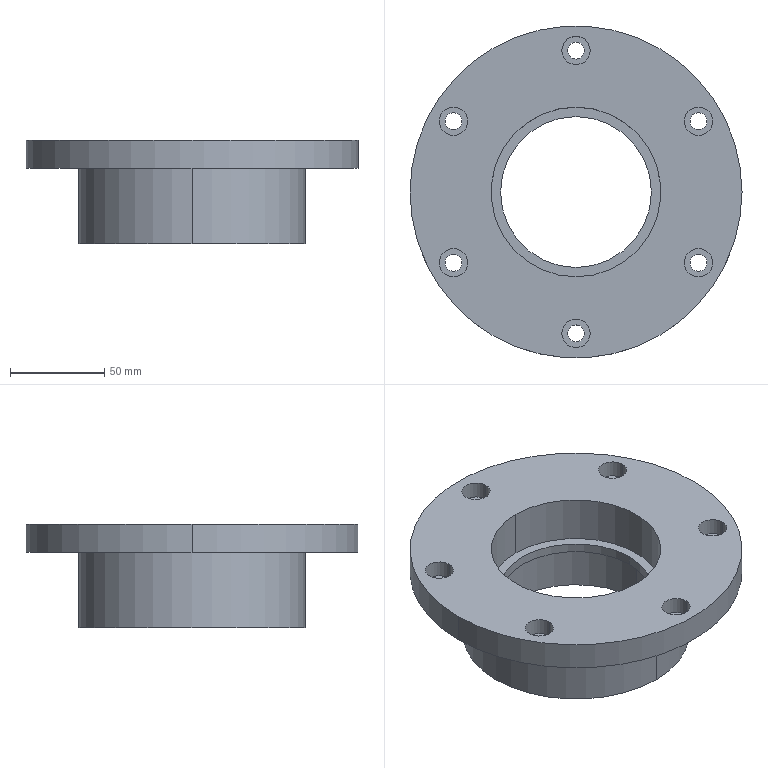Part | SolidWorks | features BaseBody 1 | 1 solid | 45 faces | box 176 x 176 x 55 mm | volume 462265 mm3 | cylinder 34 | plane 11 | commonest cylinder face diameters 9 x12 15 x12 90 x4 80 x2 120 x2 176 x2
STEP:
#1=CARTESIAN_POINT('',(72.452,37.5,46.));
#2=VERTEX_POINT('',#1);
#3=CARTESIAN_POINT('',(57.452,37.5,46.));
#4=VERTEX_POINT('',#3);
#5=CARTESIAN_POINT('',(64.952,37.5,46.));
#6=DIRECTION('',(0.,0.,-1.));
#7=DIRECTION('',(1.,0.,0.));
#8=AXIS2_PLACEMENT_3D('',#5,#6,#7);
#9=CIRCLE('',#8,7.5);
#10=EDGE_CURVE('',#2,#4,#9,.T.);
#11=ORIENTED_EDGE('',*,*,#10,.T.);
#12=CARTESIAN_POINT('',(57.452,37.5,55.));
#13=VERTEX_POINT('',#12);
#14=CARTESIAN_POINT('',(57.452,37.5,46.));
#15=DIRECTION('',(0.,0.,1.));
#16=VECTOR('',#15,1000.);
#17=LINE('',#14,#16);
#18=EDGE_CURVE('',#4,#13,#17,.T.);
#19=ORIENTED_EDGE('',*,*,#18,.T.);
#20=CARTESIAN_POINT('',(72.452,37.5,55.));
#21=VERTEX_POINT('',#20);
#22=CARTESIAN_POINT('',(64.952,37.5,55.));
#23=DIRECTION('',(0.,0.,1.));
#24=DIRECTION('',(1.,0.,0.));
#25=AXIS2_PLACEMENT_3D('',#22,#23,#24);
#26=CIRCLE('',#25,7.5);
#27=EDGE_CURVE('',#13,#21,#26,.T.);
#28=ORIENTED_EDGE('',*,*,#27,.T.);
#29=CARTESIAN_POINT('',(72.452,37.5,46.));
#30=DIRECTION('',(0.,0.,1.));
#31=VECTOR('',#30,1000.);
#32=LINE('',#29,#31);
#33=EDGE_CURVE('',#2,#21,#32,.T.);
#34=ORIENTED_EDGE('',*,*,#33,.F.);
#35=EDGE_LOOP('',(#11,#19,#28,#34));
#36=FACE_OUTER_BOUND('',#35,.T.);
#37=CARTESIAN_POINT('',(64.952,37.5,46.));
#38=DIRECTION('',(0.,0.,1.));
#39=DIRECTION('',(1.,0.,0.));
#40=AXIS2_PLACEMENT_3D('',#37,#38,#39);
#41=CYLINDRICAL_SURFACE('',#40,7.5);
#42=ADVANCED_FACE('',(#36),#41,.F.);
#43=CARTESIAN_POINT('',(0.,-45.,30.));
#44=VERTEX_POINT('',#43);
#45=CARTESIAN_POINT('',(0.,45.,30.));
#46=VERTEX_POINT('',#45);
#47=CARTESIAN_POINT('',(0.,0.,30.));
#48=DIRECTION('',(0.,0.,-1.));
#49=DIRECTION('',(0.,-1.,0.));
#50=AXIS2_PLACEMENT_3D('',#47,#48,#49);
#51=CIRCLE('',#50,45.);
#52=EDGE_CURVE('',#44,#46,#51,.T.);
#53=ORIENTED_EDGE('',*,*,#52,.T.);
#54=CARTESIAN_POINT('',(0.,45.,55.));
#55=VERTEX_POINT('',#54);
#56=CARTESIAN_POINT('',(0.,45.,30.));
#57=DIRECTION('',(0.,0.,1.));
#58=VECTOR('',#57,1000.);
#59=LINE('',#56,#58);
#60=EDGE_CURVE('',#46,#55,#59,.T.);
#61=ORIENTED_EDGE('',*,*,#60,.T.);
#62=CARTESIAN_POINT('',(0.,-45.,55.));
#63=VERTEX_POINT('',#62);
#64=CARTESIAN_POINT('',(0.,0.,55.));
#65=DIRECTION('',(0.,0.,-1.));
#66=DIRECTION('',(0.,-1.,0.));
#67=AXIS2_PLACEMENT_3D('',#64,#65,#66);
#68=CIRCLE('',#67,45.);
#69=EDGE_CURVE('',#63,#55,#68,.T.);
#70=ORIENTED_EDGE('',*,*,#69,.F.);
#71=CARTESIAN_POINT('',(0.,-45.,30.));
#72=DIRECTION('',(0.,0.,1.));
#73=VECTOR('',#72,1000.);
#74=LINE('',#71,#73);
#75=EDGE_CURVE('',#44,#63,#74,.T.);
#76=ORIENTED_EDGE('',*,*,#75,.F.);
#77=EDGE_LOOP('',(#53,#61,#70,#76));
#78=FACE_OUTER_BOUND('',#77,.T.);
#79=CARTESIAN_POINT('',(0.,0.,30.));
#80=DIRECTION('',(0.,0.,1.));
#81=DIRECTION('',(0.,-1.,0.));
#82=AXIS2_PLACEMENT_3D('',#79,#80,#81);
#83=CYLINDRICAL_SURFACE('',#82,45.);
#84=ADVANCED_FACE('',(#78),#83,.F.);
#85=CARTESIAN_POINT('',(7.5,75.,46.));
#86=VERTEX_POINT('',#85);
#87=CARTESIAN_POINT('',(-7.5,75.,46.));
#88=VERTEX_POINT('',#87);
#89=CARTESIAN_POINT('',(0.,75.,46.));
#90=DIRECTION('',(0.,0.,-1.));
#91=DIRECTION('',(1.,0.,0.));
#92=AXIS2_PLACEMENT_3D('',#89,#90,#91);
#93=CIRCLE('',#92,7.5);
#94=EDGE_CURVE('',#86,#88,#93,.T.);
#95=ORIENTED_EDGE('',*,*,#94,.T.);
#96=CARTESIAN_POINT('',(-7.5,75.,55.));
#97=VERTEX_POINT('',#96);
#98=CARTESIAN_POINT('',(-7.5,75.,46.));
#99=DIRECTION('',(0.,0.,1.));
#100=VECTOR('',#99,1000.);
#101=LINE('',#98,#100);
#102=EDGE_CURVE('',#88,#97,#101,.T.);
#103=ORIENTED_EDGE('',*,*,#102,.T.);
#104=CARTESIAN_POINT('',(7.5,75.,55.));
#105=VERTEX_POINT('',#104);
#106=CARTESIAN_POINT('',(0.,75.,55.));
#107=DIRECTION('',(0.,0.,-1.));
#108=DIRECTION('',(1.,0.,0.));
#109=AXIS2_PLACEMENT_3D('',#106,#107,#108);
#110=CIRCLE('',#109,7.5);
#111=EDGE_CURVE('',#105,#97,#110,.T.);
#112=ORIENTED_EDGE('',*,*,#111,.F.);
#113=CARTESIAN_POINT('',(7.5,75.,46.));
#114=DIRECTION('',(0.,0.,1.));
#115=VECTOR('',#114,1000.);
#116=LINE('',#113,#115);
#117=EDGE_CURVE('',#86,#105,#116,.T.);
#118=ORIENTED_EDGE('',*,*,#117,.F.);
#119=EDGE_LOOP('',(#95,#103,#112,#118));
#120=FACE_OUTER_BOUND('',#119,.T.);
#121=CARTESIAN_POINT('',(0.,75.,46.));
#122=DIRECTION('',(0.,0.,1.));
#123=DIRECTION('',(1.,0.,0.));
#124=AXIS2_PLACEMENT_3D('',#121,#122,#123);
#125=CYLINDRICAL_SURFACE('',#124,7.5);
#126=ADVANCED_FACE('',(#120),#125,.F.);
#127=CARTESIAN_POINT('',(-57.452,37.5,46.));
#128=VERTEX_POINT('',#127);
#129=CARTESIAN_POINT('',(-72.452,37.5,46.));
#130=VERTEX_POINT('',#129);
#131=CARTESIAN_POINT('',(-64.952,37.5,46.));
#132=DIRECTION('',(0.,0.,-1.));
#133=DIRECTION('',(1.,0.,0.));
#134=AXIS2_PLACEMENT_3D('',#131,#132,#133);
#135=CIRCLE('',#134,7.5);
#136=EDGE_CURVE('',#128,#130,#135,.T.);
#137=ORIENTED_EDGE('',*,*,#136,.T.);
#138=CARTESIAN_POINT('',(-72.452,37.5,55.));
#139=VERTEX_POINT('',#138);
#140=CARTESIAN_POINT('',(-72.452,37.5,46.));
#141=DIRECTION('',(0.,0.,1.));
#142=VECTOR('',#141,1000.);
#143=LINE('',#140,#142);
#144=EDGE_CURVE('',#130,#139,#143,.T.);
#145=ORIENTED_EDGE('',*,*,#144,.T.);
#146=CARTESIAN_POINT('',(-57.452,37.5,55.));
#147=VERTEX_POINT('',#146);
#148=CARTESIAN_POINT('',(-64.952,37.5,55.));
#149=DIRECTION('',(0.,0.,-1.));
#150=DIRECTION('',(1.,0.,0.));
#151=AXIS2_PLACEMENT_3D('',#148,#149,#150);
#152=CIRCLE('',#151,7.5);
#153=EDGE_CURVE('',#147,#139,#152,.T.);
#154=ORIENTED_EDGE('',*,*,#153,.F.);
#155=CARTESIAN_POINT('',(-57.452,37.5,46.));
#156=DIRECTION('',(0.,0.,1.));
#157=VECTOR('',#156,1000.);
#158=LINE('',#155,#157);
#159=EDGE_CURVE('',#128,#147,#158,.T.);
#160=ORIENTED_EDGE('',*,*,#159,.F.);
#161=EDGE_LOOP('',(#137,#145,#154,#160));
#162=FACE_OUTER_BOUND('',#161,.T.);
#163=CARTESIAN_POINT('',(-64.952,37.5,46.));
#164=DIRECTION('',(0.,0.,1.));
#165=DIRECTION('',(1.,0.,0.));
#166=AXIS2_PLACEMENT_3D('',#163,#164,#165);
#167=CYLINDRICAL_SURFACE('',#166,7.5);
#168=ADVANCED_FACE('',(#162),#167,.F.);
#169=CARTESIAN_POINT('',(-57.452,-37.5,46.));
#170=VERTEX_POINT('',#169);
#171=CARTESIAN_POINT('',(-72.452,-37.5,46.));
#172=VERTEX_POINT('',#171);
#173=CARTESIAN_POINT('',(-64.952,-37.5,46.));
#174=DIRECTION('',(0.,0.,-1.));
#175=DIRECTION('',(1.,0.,0.));
#176=AXIS2_PLACEMENT_3D('',#173,#174,#175);
#177=CIRCLE('',#176,7.5);
#178=EDGE_CURVE('',#170,#172,#177,.T.);
#179=ORIENTED_EDGE('',*,*,#178,.T.);
#180=CARTESIAN_POINT('',(-72.452,-37.5,55.));
#181=VERTEX_POINT('',#180);
#182=CARTESIAN_POINT('',(-72.452,-37.5,46.));
#183=DIRECTION('',(0.,0.,1.));
#184=VECTOR('',#183,1000.);
#185=LINE('',#182,#184);
#186=EDGE_CURVE('',#172,#181,#185,.T.);
#187=ORIENTED_EDGE('',*,*,#186,.T.);
#188=CARTESIAN_POINT('',(-57.452,-37.5,55.));
#189=VERTEX_POINT('',#188);
#190=CARTESIAN_POINT('',(-64.952,-37.5,55.));
#191=DIRECTION('',(0.,0.,-1.));
#192=DIRECTION('',(1.,0.,0.));
#193=AXIS2_PLACEMENT_3D('',#190,#191,#192);
#194=CIRCLE('',#193,7.5);
#195=EDGE_CURVE('',#189,#181,#194,.T.);
#196=ORIENTED_EDGE('',*,*,#195,.F.);
#197=CARTESIAN_POINT('',(-57.452,-37.5,46.));
#198=DIRECTION('',(0.,0.,1.));
#199=VECTOR('',#198,1000.);
#200=LINE('',#197,#199);
#201=EDGE_CURVE('',#170,#189,#200,.T.);
#202=ORIENTED_EDGE('',*,*,#201,.F.);
#203=EDGE_LOOP('',(#179,#187,#196,#202));
#204=FACE_OUTER_BOUND('',#203,.T.);
#205=CARTESIAN_POINT('',(-64.952,-37.5,46.));
#206=DIRECTION('',(0.,0.,1.));
#207=DIRECTION('',(1.,0.,0.));
#208=AXIS2_PLACEMENT_3D('',#205,#206,#207);
#209=CYLINDRICAL_SURFACE('',#208,7.5);
#210=ADVANCED_FACE('',(#204),#209,.F.);
#211=CARTESIAN_POINT('',(7.5,-75.,46.));
#212=VERTEX_POINT('',#211);
#213=CARTESIAN_POINT('',(-7.5,-75.,46.));
#214=VERTEX_POINT('',#213);
#215=CARTESIAN_POINT('',(0.,-75.,46.));
#216=DIRECTION('',(0.,0.,-1.));
#217=DIRECTION('',(1.,0.,0.));
#218=AXIS2_PLACEMENT_3D('',#215,#216,#217);
#219=CIRCLE('',#218,7.5);
#220=EDGE_CURVE('',#212,#214,#219,.T.);
#221=ORIENTED_EDGE('',*,*,#220,.T.);
#222=CARTESIAN_POINT('',(-7.5,-75.,55.));
#223=VERTEX_POINT('',#222);
#224=CARTESIAN_POINT('',(-7.5,-75.,46.));
#225=DIRECTION('',(0.,0.,1.));
#226=VECTOR('',#225,1000.);
#227=LINE('',#224,#226);
#228=EDGE_CURVE('',#214,#223,#227,.T.);
#229=ORIENTED_EDGE('',*,*,#228,.T.);
#230=CARTESIAN_POINT('',(7.5,-75.,55.));
#231=VERTEX_POINT('',#230);
#232=CARTESIAN_POINT('',(0.,-75.,55.));
#233=DIRECTION('',(0.,0.,-1.));
#234=DIRECTION('',(1.,0.,0.));
#235=AXIS2_PLACEMENT_3D('',#232,#233,#234);
#236=CIRCLE('',#235,7.5);
#237=EDGE_CURVE('',#231,#223,#236,.T.);
#238=ORIENTED_EDGE('',*,*,#237,.F.);
#239=CARTESIAN_POINT('',(7.5,-75.,46.));
#240=DIRECTION('',(0.,0.,1.));
#241=VECTOR('',#240,1000.);
#242=LINE('',#239,#241);
#243=EDGE_CURVE('',#212,#231,#242,.T.);
#244=ORIENTED_EDGE('',*,*,#243,.F.);
#245=EDGE_LOOP('',(#221,#229,#238,#244));
#246=FACE_OUTER_BOUND('',#245,.T.);
#247=CARTESIAN_POINT('',(0.,-75.,46.));
#248=DIRECTION('',(0.,0.,1.));
#249=DIRECTION('',(1.,0.,0.));
#250=AXIS2_PLACEMENT_3D('',#247,#248,#249);
#251=CYLINDRICAL_SURFACE('',#250,7.5);
#252=ADVANCED_FACE('',(#246),#251,.F.);
#253=CARTESIAN_POINT('',(72.452,-37.5,46.));
#254=VERTEX_POINT('',#253);
#255=CARTESIAN_POINT('',(57.452,-37.5,46.));
#256=VERTEX_POINT('',#255);
#257=CARTESIAN_POINT('',(64.952,-37.5,46.));
#258=DIRECTION('',(0.,0.,-1.));
#259=DIRECTION('',(1.,0.,0.));
#260=AXIS2_PLACEMENT_3D('',#257,#258,#259);
#261=CIRCLE('',#260,7.5);
#262=EDGE_CURVE('',#254,#256,#261,.T.);
#263=ORIENTED_EDGE('',*,*,#262,.T.);
#264=CARTESIAN_POINT('',(57.452,-37.5,55.));
#265=VERTEX_POINT('',#264);
#266=CARTESIAN_POINT('',(57.452,-37.5,46.));
#267=DIRECTION('',(0.,0.,1.));
#268=VECTOR('',#267,1000.);
#269=LINE('',#266,#268);
#270=EDGE_CURVE('',#256,#265,#269,.T.);
#271=ORIENTED_EDGE('',*,*,#270,.T.);
#272=CARTESIAN_POINT('',(72.452,-37.5,55.));
#273=VERTEX_POINT('',#272);
#274=CARTESIAN_POINT('',(64.952,-37.5,55.));
#275=DIRECTION('',(0.,0.,-1.));
#276=DIRECTION('',(1.,0.,0.));
#277=AXIS2_PLACEMENT_3D('',#274,#275,#276);
#278=CIRCLE('',#277,7.5);
#279=EDGE_CURVE('',#273,#265,#278,.T.);
#280=ORIENTED_EDGE('',*,*,#279,.F.);
#281=CARTESIAN_POINT('',(72.452,-37.5,46.));
#282=DIRECTION('',(0.,0.,1.));
#283=VECTOR('',#282,1000.);
#284=LINE('',#281,#283);
#285=EDGE_CURVE('',#254,#273,#284,.T.);
#286=ORIENTED_EDGE('',*,*,#285,.F.);
#287=EDGE_LOOP('',(#263,#271,#280,#286));
#288=FACE_OUTER_BOUND('',#287,.T.);
#289=CARTESIAN_POINT('',(64.952,-37.5,46.));
#290=DIRECTION('',(0.,0.,1.));
#291=DIRECTION('',(1.,0.,0.));
#292=AXIS2_PLACEMENT_3D('',#289,#290,#291);
#293=CYLINDRICAL_SURFACE('',#292,7.5);
#294=ADVANCED_FACE('',(#288),#293,.F.);
#295=CARTESIAN_POINT('',(88.,0.,55.));
#296=VERTEX_POINT('',#295);
#297=CARTESIAN_POINT('',(-88.,0.,55.));
#298=VERTEX_POINT('',#297);
#299=CARTESIAN_POINT('',(0.,0.,55.));
#300=DIRECTION('',(0.,0.,1.));
#301=DIRECTION('',(-1.,0.,0.));
#302=AXIS2_PLACEMENT_3D('',#299,#300,#301);
#303=CIRCLE('',#302,88.);
#304=EDGE_CURVE('',#296,#298,#303,.T.);
#305=ORIENTED_EDGE('',*,*,#304,.F.);
#306=CARTESIAN_POINT('',(88.,0.,40.));
#307=VERTEX_POINT('',#306);
#308=CARTESIAN_POINT('',(88.,0.,55.));
#309=DIRECTION('',(0.,0.,-1.));
#310=VECTOR('',#309,1000.);
#311=LINE('',#308,#310);
#312=EDGE_CURVE('',#296,#307,#311,.T.);
#313=ORIENTED_EDGE('',*,*,#312,.T.);
#314=CARTESIAN_POINT('',(-88.,0.,40.));
#315=VERTEX_POINT('',#314);
#316=CARTESIAN_POINT('',(0.,0.,40.));
#317=DIRECTION('',(0.,0.,-1.));
#318=DIRECTION('',(-1.,0.,0.));
#319=AXIS2_PLACEMENT_3D('',#316,#317,#318);
#320=CIRCLE('',#319,88.);
#321=EDGE_CURVE('',#315,#307,#320,.T.);
#322=ORIENTED_EDGE('',*,*,#321,.F.);
#323=CARTESIAN_POINT('',(-88.,0.,55.));
#324=DIRECTION('',(0.,0.,-1.));
#325=VECTOR('',#324,1000.);
#326=LINE('',#323,#325);
#327=EDGE_CURVE('',#298,#315,#326,.T.);
#328=ORIENTED_EDGE('',*,*,#327,.F.);
#329=EDGE_LOOP('',(#305,#313,#322,#328));
#330=FACE_OUTER_BOUND('',#329,.T.);
#331=CARTESIAN_POINT('',(0.,0.,55.));
#332=DIRECTION('',(0.,0.,-1.));
#333=DIRECTION('',(-1.,0.,0.));
#334=AXIS2_PLACEMENT_3D('',#331,#332,#333);
#335=CYLINDRICAL_SURFACE('',#334,88.);
#336=ADVANCED_FACE('',(#330),#335,.T.);
#337=CARTESIAN_POINT('',(64.952,33.,40.));
#338=VERTEX_POINT('',#337);
#339=CARTESIAN_POINT('',(64.952,42.,40.));
#340=VERTEX_POINT('',#339);
#341=CARTESIAN_POINT('',(64.952,37.5,40.));
#342=DIRECTION('',(0.,0.,-1.));
#343=DIRECTION('',(0.,-1.,0.));
#344=AXIS2_PLACEMENT_3D('',#341,#342,#343);
#345=CIRCLE('',#344,4.5);
#346=EDGE_CURVE('',#338,#340,#345,.T.);
#347=ORIENTED_EDGE('',*,*,#346,.T.);
#348=CARTESIAN_POINT('',(64.952,42.,46.));
#349=VERTEX_POINT('',#348);
#350=CARTESIAN_POINT('',(64.952,42.,40.));
#351=DIRECTION('',(0.,0.,1.));
#352=VECTOR('',#351,1000.);
#353=LINE('',#350,#352);
#354=EDGE_CURVE('',#340,#349,#353,.T.);
#355=ORIENTED_EDGE('',*,*,#354,.T.);
#356=CARTESIAN_POINT('',(64.952,33.,46.));
#357=VERTEX_POINT('',#356);
#358=CARTESIAN_POINT('',(64.952,37.5,46.));
#359=DIRECTION('',(0.,0.,1.));
#360=DIRECTION('',(0.,-1.,0.));
#361=AXIS2_PLACEMENT_3D('',#358,#359,#360);
#362=CIRCLE('',#361,4.5);
#363=EDGE_CURVE('',#349,#357,#362,.T.);
#364=ORIENTED_EDGE('',*,*,#363,.T.);
#365=CARTESIAN_POINT('',(64.952,33.,40.));
#366=DIRECTION('',(0.,0.,1.));
#367=VECTOR('',#366,1000.);
#368=LINE('',#365,#367);
#369=EDGE_CURVE('',#338,#357,#368,.T.);
#370=ORIENTED_EDGE('',*,*,#369,.F.);
#371=EDGE_LOOP('',(#347,#355,#364,#370));
#372=FACE_OUTER_BOUND('',#371,.T.);
#373=CARTESIAN_POINT('',(64.952,37.5,40.));
#374=DIRECTION('',(0.,0.,1.));
#375=DIRECTION('',(0.,-1.,0.));
#376=AXIS2_PLACEMENT_3D('',#373,#374,#375);
#377=CYLINDRICAL_SURFACE('',#376,4.5);
#378=ADVANCED_FACE('',(#372),#377,.F.);
#379=CARTESIAN_POINT('',(40.,0.,25.));
#380=VERTEX_POINT('',#379);
#381=CARTESIAN_POINT('',(-40.,0.,25.));
#382=VERTEX_POINT('',#381);
#383=CARTESIAN_POINT('',(0.,0.,25.));
#384=DIRECTION('',(0.,0.,-1.));
#385=DIRECTION('',(1.,0.,0.));
#386=AXIS2_PLACEMENT_3D('',#383,#384,#385);
#387=CIRCLE('',#386,40.);
#388=EDGE_CURVE('',#380,#382,#387,.T.);
#389=ORIENTED_EDGE('',*,*,#388,.T.);
#390=CARTESIAN_POINT('',(-40.,0.,30.));
#391=VERTEX_POINT('',#390);
#392=CARTESIAN_POINT('',(-40.,0.,25.));
#393=DIRECTION('',(0.,0.,1.));
#394=VECTOR('',#393,1000.);
#395=LINE('',#392,#394);
#396=EDGE_CURVE('',#382,#391,#395,.T.);
#397=ORIENTED_EDGE('',*,*,#396,.T.);
#398=CARTESIAN_POINT('',(40.,0.,30.));
#399=VERTEX_POINT('',#398);
#400=CARTESIAN_POINT('',(0.,0.,30.));
#401=DIRECTION('',(0.,0.,-1.));
#402=DIRECTION('',(1.,0.,0.));
#403=AXIS2_PLACEMENT_3D('',#400,#401,#402);
#404=CIRCLE('',#403,40.);
#405=EDGE_CURVE('',#399,#391,#404,.T.);
#406=ORIENTED_EDGE('',*,*,#405,.F.);
#407=CARTESIAN_POINT('',(40.,0.,25.));
#408=DIRECTION('',(0.,0.,1.));
#409=VECTOR('',#408,1000.);
#410=LINE('',#407,#409);
#411=EDGE_CURVE('',#380,#399,#410,.T.);
#412=ORIENTED_EDGE('',*,*,#411,.F.);
#413=EDGE_LOOP('',(#389,#397,#406,#412));
#414=FACE_OUTER_BOUND('',#413,.T.);
#415=CARTESIAN_POINT('',(0.,0.,25.));
#416=DIRECTION('',(0.,0.,1.));
#417=DIRECTION('',(1.,0.,0.));
#418=AXIS2_PLACEMENT_3D('',#415,#416,#417);
#419=CYLINDRICAL_SURFACE('',#418,40.);
#420=ADVANCED_FACE('',(#414),#419,.F.);
#421=CARTESIAN_POINT('',(0.,70.5,40.));
#422=VERTEX_POINT('',#421);
#423=CARTESIAN_POINT('',(0.,79.5,40.));
#424=VERTEX_POINT('',#423);
#425=CARTESIAN_POINT('',(0.,75.,40.));
#426=DIRECTION('',(0.,0.,-1.));
#427=DIRECTION('',(0.,-1.,0.));
#428=AXIS2_PLACEMENT_3D('',#425,#426,#427);
#429=CIRCLE('',#428,4.5);
#430=EDGE_CURVE('',#422,#424,#429,.T.);
#431=ORIENTED_EDGE('',*,*,#430,.T.);
#432=CARTESIAN_POINT('',(0.,79.5,46.));
#433=VERTEX_POINT('',#432);
#434=CARTESIAN_POINT('',(0.,79.5,40.));
#435=DIRECTION('',(0.,0.,1.));
#436=VECTOR('',#435,1000.);
#437=LINE('',#434,#436);
#438=EDGE_CURVE('',#424,#433,#437,.T.);
#439=ORIENTED_EDGE('',*,*,#438,.T.);
#440=CARTESIAN_POINT('',(0.,70.5,46.));
#441=VERTEX_POINT('',#440);
#442=CARTESIAN_POINT('',(0.,75.,46.));
#443=DIRECTION('',(0.,0.,1.));
#444=DIRECTION('',(0.,-1.,0.));
#445=AXIS2_PLACEMENT_3D('',#442,#443,#444);
#446=CIRCLE('',#445,4.5);
#447=EDGE_CURVE('',#433,#441,#446,.T.);
#448=ORIENTED_EDGE('',*,*,#447,.T.);
#449=CARTESIAN_POINT('',(0.,70.5,40.));
#450=DIRECTION('',(0.,0.,1.));
#451=VECTOR('',#450,1000.);
#452=LINE('',#449,#451);
#453=EDGE_CURVE('',#422,#441,#452,.T.);
#454=ORIENTED_EDGE('',*,*,#453,.F.);
#455=EDGE_LOOP('',(#431,#439,#448,#454));
#456=FACE_OUTER_BOUND('',#455,.T.);
#457=CARTESIAN_POINT('',(0.,75.,40.));
#458=DIRECTION('',(0.,0.,1.));
#459=DIRECTION('',(0.,-1.,0.));
#460=AXIS2_PLACEMENT_3D('',#457,#458,#459);
#461=CYLINDRICAL_SURFACE('',#460,4.5);
#462=ADVANCED_FACE('',(#456),#461,.F.);
#463=CARTESIAN_POINT('',(-64.952,33.,40.));
#464=VERTEX_POINT('',#463);
#465=CARTESIAN_POINT('',(-64.952,42.,40.));
#466=VERTEX_POINT('',#465);
#467=CARTESIAN_POINT('',(-64.952,37.5,40.));
#468=DIRECTION('',(0.,0.,-1.));
#469=DIRECTION('',(0.,-1.,0.));
#470=AXIS2_PLACEMENT_3D('',#467,#468,#469);
#471=CIRCLE('',#470,4.5);
#472=EDGE_CURVE('',#464,#466,#471,.T.);
#473=ORIENTED_EDGE('',*,*,#472,.T.);
#474=CARTESIAN_POINT('',(-64.952,42.,46.));
#475=VERTEX_POINT('',#474);
#476=CARTESIAN_POINT('',(-64.952,42.,40.));
#477=DIRECTION('',(0.,0.,1.));
#478=VECTOR('',#477,1000.);
#479=LINE('',#476,#478);
#480=EDGE_CURVE('',#466,#475,#479,.T.);
#481=ORIENTED_EDGE('',*,*,#480,.T.);
#482=CARTESIAN_POINT('',(-64.952,33.,46.));
#483=VERTEX_POINT('',#482);
#484=CARTESIAN_POINT('',(-64.952,37.5,46.));
#485=DIRECTION('',(0.,0.,1.));
#486=DIRECTION('',(0.,-1.,0.));
#487=AXIS2_PLACEMENT_3D('',#484,#485,#486);
#488=CIRCLE('',#487,4.5);
#489=EDGE_CURVE('',#475,#483,#488,.T.);
#490=ORIENTED_EDGE('',*,*,#489,.T.);
#491=CARTESIAN_POINT('',(-64.952,33.,40.));
#492=DIRECTION('',(0.,0.,1.));
#493=VECTOR('',#492,1000.);
#494=LINE('',#491,#493);
#495=EDGE_CURVE('',#464,#483,#494,.T.);
#496=ORIENTED_EDGE('',*,*,#495,.F.);
#497=EDGE_LOOP('',(#473,#481,#490,#496));
#498=FACE_OUTER_BOUND('',#497,.T.);
#499=CARTESIAN_POINT('',(-64.952,37.5,40.));
#500=DIRECTION('',(0.,0.,1.));
#501=DIRECTION('',(0.,-1.,0.));
#502=AXIS2_PLACEMENT_3D('',#499,#500,#501);
#503=CYLINDRICAL_SURFACE('',#502,4.5);
#504=ADVANCED_FACE('',(#498),#503,.F.);
#505=CARTESIAN_POINT('',(-64.952,-42.,40.));
#506=VERTEX_POINT('',#505);
#507=CARTESIAN_POINT('',(-64.952,-33.,40.));
#508=VERTEX_POINT('',#507);
#509=CARTESIAN_POINT('',(-64.952,-37.5,40.));
#510=DIRECTION('',(0.,0.,-1.));
#511=DIRECTION('',(0.,-1.,0.));
#512=AXIS2_PLACEMENT_3D('',#509,#510,#511);
#513=CIRCLE('',#512,4.5);
#514=EDGE_CURVE('',#506,#508,#513,.T.);
#515=ORIENTED_EDGE('',*,*,#514,.T.);
#516=CARTESIAN_POINT('',(-64.952,-33.,46.));
#517=VERTEX_POINT('',#516);
#518=CARTESIAN_POINT('',(-64.952,-33.,40.));
#519=DIRECTION('',(0.,0.,1.));
#520=VECTOR('',#519,1000.);
#521=LINE('',#518,#520);
#522=EDGE_CURVE('',#508,#517,#521,.T.);
#523=ORIENTED_EDGE('',*,*,#522,.T.);
#524=CARTESIAN_POINT('',(-64.952,-42.,46.));
#525=VERTEX_POINT('',#524);
#526=CARTESIAN_POINT('',(-64.952,-37.5,46.));
#527=DIRECTION('',(0.,0.,1.));
#528=DIRECTION('',(0.,-1.,0.));
#529=AXIS2_PLACEMENT_3D('',#526,#527,#528);
#530=CIRCLE('',#529,4.5);
#531=EDGE_CURVE('',#517,#525,#530,.T.);
#532=ORIENTED_EDGE('',*,*,#531,.T.);
#533=CARTESIAN_POINT('',(-64.952,-42.,40.));
#534=DIRECTION('',(0.,0.,1.));
#535=VECTOR('',#534,1000.);
#536=LINE('',#533,#535);
#537=EDGE_CURVE('',#506,#525,#536,.T.);
#538=ORIENTED_EDGE('',*,*,#537,.F.);
#539=EDGE_LOOP('',(#515,#523,#532,#538));
#540=FACE_OUTER_BOUND('',#539,.T.);
#541=CARTESIAN_POINT('',(-64.952,-37.5,40.));
#542=DIRECTION('',(0.,0.,1.));
#543=DIRECTION('',(0.,-1.,0.));
#544=AXIS2_PLACEMENT_3D('',#541,#542,#543);
#545=CYLINDRICAL_SURFACE('',#544,4.5);
#546=ADVANCED_FACE('',(#540),#545,.F.);
#547=CARTESIAN_POINT('',(0.,-79.5,40.));
#548=VERTEX_POINT('',#547);
#549=CARTESIAN_POINT('',(0.,-70.5,40.));
#550=VERTEX_POINT('',#549);
#551=CARTESIAN_POINT('',(0.,-75.,40.));
#552=DIRECTION('',(0.,0.,-1.));
#553=DIRECTION('',(0.,-1.,0.));
#554=AXIS2_PLACEMENT_3D('',#551,#552,#553);
#555=CIRCLE('',#554,4.5);
#556=EDGE_CURVE('',#548,#550,#555,.T.);
#557=ORIENTED_EDGE('',*,*,#556,.T.);
#558=CARTESIAN_POINT('',(0.,-70.5,46.));
#559=VERTEX_POINT('',#558);
#560=CARTESIAN_POINT('',(0.,-70.5,40.));
#561=DIRECTION('',(0.,0.,1.));
#562=VECTOR('',#561,1000.);
#563=LINE('',#560,#562);
#564=EDGE_CURVE('',#550,#559,#563,.T.);
#565=ORIENTED_EDGE('',*,*,#564,.T.);
#566=CARTESIAN_POINT('',(0.,-79.5,46.));
#567=VERTEX_POINT('',#566);
#568=CARTESIAN_POINT('',(0.,-75.,46.));
#569=DIRECTION('',(0.,0.,1.));
#570=DIRECTION('',(0.,-1.,0.));
#571=AXIS2_PLACEMENT_3D('',#568,#569,#570);
#572=CIRCLE('',#571,4.5);
#573=EDGE_CURVE('',#559,#567,#572,.T.);
#574=ORIENTED_EDGE('',*,*,#573,.T.);
#575=CARTESIAN_POINT('',(0.,-79.5,40.));
#576=DIRECTION('',(0.,0.,1.));
#577=VECTOR('',#576,1000.);
#578=LINE('',#575,#577);
#579=EDGE_CURVE('',#548,#567,#578,.T.);
#580=ORIENTED_EDGE('',*,*,#579,.F.);
#581=EDGE_LOOP('',(#557,#565,#574,#580));
#582=FACE_OUTER_BOUND('',#581,.T.);
#583=CARTESIAN_POINT('',(0.,-75.,40.));
#584=DIRECTION('',(0.,0.,1.));
#585=DIRECTION('',(0.,-1.,0.));
#586=AXIS2_PLACEMENT_3D('',#583,#584,#585);
#587=CYLINDRICAL_SURFACE('',#586,4.5);
#588=ADVANCED_FACE('',(#582),#587,.F.);
#589=CARTESIAN_POINT('',(64.952,-42.,40.));
#590=VERTEX_POINT('',#589);
#591=CARTESIAN_POINT('',(64.952,-33.,40.));
#592=VERTEX_POINT('',#591);
#593=CARTESIAN_POINT('',(64.952,-37.5,40.));
#594=DIRECTION('',(0.,0.,-1.));
#595=DIRECTION('',(0.,-1.,0.));
#596=AXIS2_PLACEMENT_3D('',#593,#594,#595);
#597=CIRCLE('',#596,4.5);
#598=EDGE_CURVE('',#590,#592,#597,.T.);
#599=ORIENTED_EDGE('',*,*,#598,.T.);
#600=CARTESIAN_POINT('',(64.952,-33.,46.));
#601=VERTEX_POINT('',#600);
#602=CARTESIAN_POINT('',(64.952,-33.,40.));
#603=DIRECTION('',(0.,0.,1.));
#604=VECTOR('',#603,1000.);
#605=LINE('',#602,#604);
#606=EDGE_CURVE('',#592,#601,#605,.T.);
#607=ORIENTED_EDGE('',*,*,#606,.T.);
#608=CARTESIAN_POINT('',(64.952,-42.,46.));
#609=VERTEX_POINT('',#608);
#610=CARTESIAN_POINT('',(64.952,-37.5,46.));
#611=DIRECTION('',(0.,0.,1.));
#612=DIRECTION('',(0.,-1.,0.));
#613=AXIS2_PLACEMENT_3D('',#610,#611,#612);
#614=CIRCLE('',#613,4.5);
#615=EDGE_CURVE('',#601,#609,#614,.T.);
#616=ORIENTED_EDGE('',*,*,#615,.T.);
#617=CARTESIAN_POINT('',(64.952,-42.,40.));
#618=DIRECTION('',(0.,0.,1.));
#619=VECTOR('',#618,1000.);
#620=LINE('',#617,#619);
#621=EDGE_CURVE('',#590,#609,#620,.T.);
#622=ORIENTED_EDGE('',*,*,#621,.F.);
#623=EDGE_LOOP('',(#599,#607,#616,#622));
#624=FACE_OUTER_BOUND('',#623,.T.);
#625=CARTESIAN_POINT('',(64.952,-37.5,40.));
#626=DIRECTION('',(0.,0.,1.));
#627=DIRECTION('',(0.,-1.,0.));
#628=AXIS2_PLACEMENT_3D('',#625,#626,#627);
#629=CYLINDRICAL_SURFACE('',#628,4.5);
#630=ADVANCED_FACE('',(#624),#629,.F.);
#631=CARTESIAN_POINT('',(0.,60.,40.));
#632=VERTEX_POINT('',#631);
#633=CARTESIAN_POINT('',(0.,-60.,40.));
#634=VERTEX_POINT('',#633);
#635=CARTESIAN_POINT('',(0.,0.,40.));
#636=DIRECTION('',(0.,0.,-1.));
#637=DIRECTION('',(0.,1.,0.));
#638=AXIS2_PLACEMENT_3D('',#635,#636,#637);
#639=CIRCLE('',#638,60.);
#640=EDGE_CURVE('',#632,#634,#639,.T.);
#641=ORIENTED_EDGE('',*,*,#640,.T.);
#642=CARTESIAN_POINT('',(0.,-60.,0.));
#643=VERTEX_POINT('',#642);
#644=CARTESIAN_POINT('',(0.,-60.,40.));
#645=DIRECTION('',(0.,0.,-1.));
#646=VECTOR('',#645,1000.);
#647=LINE('',#644,#646);
#648=EDGE_CURVE('',#634,#643,#647,.T.);
#649=ORIENTED_EDGE('',*,*,#648,.T.);
#650=CARTESIAN_POINT('',(0.,60.,0.));
#651=VERTEX_POINT('',#650);
#652=CARTESIAN_POINT('',(0.,0.,0.));
#653=DIRECTION('',(0.,0.,-1.));
#654=DIRECTION('',(0.,1.,0.));
#655=AXIS2_PLACEMENT_3D('',#652,#653,#654);
#656=CIRCLE('',#655,60.);
#657=EDGE_CURVE('',#651,#643,#656,.T.);
#658=ORIENTED_EDGE('',*,*,#657,.F.);
#659=CARTESIAN_POINT('',(0.,60.,40.));
#660=DIRECTION('',(0.,0.,-1.));
#661=VECTOR('',#660,1000.);
#662=LINE('',#659,#661);
#663=EDGE_CURVE('',#632,#651,#662,.T.);
#664=ORIENTED_EDGE('',*,*,#663,.F.);
#665=EDGE_LOOP('',(#641,#649,#658,#664));
#666=FACE_OUTER_BOUND('',#665,.T.);
#667=CARTESIAN_POINT('',(0.,0.,40.));
#668=DIRECTION('',(0.,0.,-1.));
#669=DIRECTION('',(0.,1.,0.));
#670=AXIS2_PLACEMENT_3D('',#667,#668,#669);
#671=CYLINDRICAL_SURFACE('',#670,60.);
#672=ADVANCED_FACE('',(#666),#671,.T.);
#673=CARTESIAN_POINT('',(45.,0.,25.));
#674=VERTEX_POINT('',#673);
#675=CARTESIAN_POINT('',(-45.,0.,25.));
#676=VERTEX_POINT('',#675);
#677=CARTESIAN_POINT('',(0.,0.,25.));
#678=DIRECTION('',(0.,0.,-1.));
#679=DIRECTION('',(-1.,0.,0.));
#680=AXIS2_PLACEMENT_3D('',#677,#678,#679);
#681=CIRCLE('',#680,45.);
#682=EDGE_CURVE('',#674,#676,#681,.T.);
#683=ORIENTED_EDGE('',*,*,#682,.F.);
#684=CARTESIAN_POINT('',(45.,0.,0.));
#685=VERTEX_POINT('',#684);
#686=CARTESIAN_POINT('',(45.,0.,25.));
#687=DIRECTION('',(0.,0.,-1.));
#688=VECTOR('',#687,1000.);
#689=LINE('',#686,#688);
#690=EDGE_CURVE('',#674,#685,#689,.T.);
#691=ORIENTED_EDGE('',*,*,#690,.T.);
#692=CARTESIAN_POINT('',(-45.,0.,0.));
#693=VERTEX_POINT('',#692);
#694=CARTESIAN_POINT('',(0.,0.,0.));
#695=DIRECTION('',(0.,0.,-1.));
#696=DIRECTION('',(-1.,0.,0.));
#697=AXIS2_PLACEMENT_3D('',#694,#695,#696);
#698=CIRCLE('',#697,45.);
#699=EDGE_CURVE('',#685,#693,#698,.T.);
#700=ORIENTED_EDGE('',*,*,#699,.T.);
#701=CARTESIAN_POINT('',(-45.,0.,25.));
#702=DIRECTION('',(0.,0.,-1.));
#703=VECTOR('',#702,1000.);
#704=LINE('',#701,#703);
#705=EDGE_CURVE('',#676,#693,#704,.T.);
#706=ORIENTED_EDGE('',*,*,#705,.F.);
#707=EDGE_LOOP('',(#683,#691,#700,#706));
#708=FACE_OUTER_BOUND('',#707,.T.);
#709=CARTESIAN_POINT('',(0.,0.,25.));
#710=DIRECTION('',(0.,0.,-1.));
#711=DIRECTION('',(-1.,0.,0.));
#712=AXIS2_PLACEMENT_3D('',#709,#710,#711);
#713=CYLINDRICAL_SURFACE('',#712,45.);
#714=ADVANCED_FACE('',(#708),#713,.F.);
#715=ORIENTED_EDGE('',*,*,#18,.F.);
#716=CARTESIAN_POINT('',(64.952,37.5,46.));
#717=DIRECTION('',(0.,0.,-1.));
#718=DIRECTION('',(1.,0.,0.));
#719=AXIS2_PLACEMENT_3D('',#716,#717,#718);
#720=CIRCLE('',#719,7.5);
#721=EDGE_CURVE('',#4,#2,#720,.T.);
#722=ORIENTED_EDGE('',*,*,#721,.T.);
#723=ORIENTED_EDGE('',*,*,#33,.T.);
#724=CARTESIAN_POINT('',(64.952,37.5,55.));
#725=DIRECTION('',(0.,0.,1.));
#726=DIRECTION('',(1.,0.,0.));
#727=AXIS2_PLACEMENT_3D('',#724,#725,#726);
#728=CIRCLE('',#727,7.5);
#729=EDGE_CURVE('',#21,#13,#728,.T.);
#730=ORIENTED_EDGE('',*,*,#729,.T.);
#731=EDGE_LOOP('',(#715,#722,#723,#730));
#732=FACE_OUTER_BOUND('',#731,.T.);
#733=CARTESIAN_POINT('',(64.952,37.5,46.));
#734=DIRECTION('',(0.,0.,1.));
#735=DIRECTION('',(1.,0.,0.));
#736=AXIS2_PLACEMENT_3D('',#733,#734,#735);
#737=CYLINDRICAL_SURFACE('',#736,7.5);
#738=ADVANCED_FACE('',(#732),#737,.F.);
#739=ORIENTED_EDGE('',*,*,#69,.T.);
#740=CARTESIAN_POINT('',(0.,0.,55.));
#741=DIRECTION('',(0.,0.,-1.));
#742=DIRECTION('',(0.,-1.,0.));
#743=AXIS2_PLACEMENT_3D('',#740,#741,#742);
#744=CIRCLE('',#743,45.);
#745=EDGE_CURVE('',#55,#63,#744,.T.);
#746=ORIENTED_EDGE('',*,*,#745,.T.);
#747=EDGE_LOOP('',(#739,#746));
#748=FACE_BOUND('',#747,.T.);
#749=ORIENTED_EDGE('',*,*,#111,.T.);
#750=CARTESIAN_POINT('',(0.,75.,55.));
#751=DIRECTION('',(0.,0.,-1.));
#752=DIRECTION('',(1.,0.,0.));
#753=AXIS2_PLACEMENT_3D('',#750,#751,#752);
#754=CIRCLE('',#753,7.5);
#755=EDGE_CURVE('',#97,#105,#754,.T.);
#756=ORIENTED_EDGE('',*,*,#755,.T.);
#757=EDGE_LOOP('',(#749,#756));
#758=FACE_BOUND('',#757,.T.);
#759=ORIENTED_EDGE('',*,*,#153,.T.);
#760=CARTESIAN_POINT('',(-64.952,37.5,55.));
#761=DIRECTION('',(0.,0.,-1.));
#762=DIRECTION('',(1.,0.,0.));
#763=AXIS2_PLACEMENT_3D('',#760,#761,#762);
#764=CIRCLE('',#763,7.5);
#765=EDGE_CURVE('',#139,#147,#764,.T.);
#766=ORIENTED_EDGE('',*,*,#765,.T.);
#767=EDGE_LOOP('',(#759,#766));
#768=FACE_BOUND('',#767,.T.);
#769=ORIENTED_EDGE('',*,*,#195,.T.);
#770=CARTESIAN_POINT('',(-64.952,-37.5,55.));
#771=DIRECTION('',(0.,0.,-1.));
#772=DIRECTION('',(1.,0.,0.));
#773=AXIS2_PLACEMENT_3D('',#770,#771,#772);
#774=CIRCLE('',#773,7.5);
#775=EDGE_CURVE('',#181,#189,#774,.T.);
#776=ORIENTED_EDGE('',*,*,#775,.T.);
#777=EDGE_LOOP('',(#769,#776));
#778=FACE_BOUND('',#777,.T.);
#779=ORIENTED_EDGE('',*,*,#237,.T.);
#780=CARTESIAN_POINT('',(0.,-75.,55.));
#781=DIRECTION('',(0.,0.,-1.));
#782=DIRECTION('',(1.,0.,0.));
#783=AXIS2_PLACEMENT_3D('',#780,#781,#782);
#784=CIRCLE('',#783,7.5);
#785=EDGE_CURVE('',#223,#231,#784,.T.);
#786=ORIENTED_EDGE('',*,*,#785,.T.);
#787=EDGE_LOOP('',(#779,#786));
#788=FACE_BOUND('',#787,.T.);
#789=ORIENTED_EDGE('',*,*,#279,.T.);
#790=CARTESIAN_POINT('',(64.952,-37.5,55.));
#791=DIRECTION('',(0.,0.,-1.));
#792=DIRECTION('',(1.,0.,0.));
#793=AXIS2_PLACEMENT_3D('',#790,#791,#792);
#794=CIRCLE('',#793,7.5);
#795=EDGE_CURVE('',#265,#273,#794,.T.);
#796=ORIENTED_EDGE('',*,*,#795,.T.);
#797=EDGE_LOOP('',(#789,#796));
#798=FACE_BOUND('',#797,.T.);
#799=ORIENTED_EDGE('',*,*,#729,.F.);
#800=ORIENTED_EDGE('',*,*,#27,.F.);
#801=EDGE_LOOP('',(#799,#800));
#802=FACE_BOUND('',#801,.T.);
#803=CARTESIAN_POINT('',(0.,0.,55.));
#804=DIRECTION('',(0.,0.,1.));
#805=DIRECTION('',(-1.,0.,0.));
#806=AXIS2_PLACEMENT_3D('',#803,#804,#805);
#807=CIRCLE('',#806,88.);
#808=EDGE_CURVE('',#298,#296,#807,.T.);
#809=ORIENTED_EDGE('',*,*,#808,.T.);
#810=ORIENTED_EDGE('',*,*,#304,.T.);
#811=EDGE_LOOP('',(#809,#810));
#812=FACE_OUTER_BOUND('',#811,.T.);
#813=CARTESIAN_POINT('',(-89.056,-89.056,55.));
#814=DIRECTION('',(0.,0.,1.));
#815=DIRECTION('',(1.,0.,0.));
#816=AXIS2_PLACEMENT_3D('',#813,#814,#815);
#817=PLANE('',#816);
#818=ADVANCED_FACE('',(#748,#758,#768,#778,#788,#798,#802,#812),#817,.T.);
#819=CARTESIAN_POINT('',(64.952,37.5,46.));
#820=DIRECTION('',(0.,0.,1.));
#821=DIRECTION('',(0.,-1.,0.));
#822=AXIS2_PLACEMENT_3D('',#819,#820,#821);
#823=CIRCLE('',#822,4.5);
#824=EDGE_CURVE('',#357,#349,#823,.T.);
#825=ORIENTED_EDGE('',*,*,#824,.F.);
#826=ORIENTED_EDGE('',*,*,#363,.F.);
#827=EDGE_LOOP('',(#825,#826));
#828=FACE_BOUND('',#827,.T.);
#829=ORIENTED_EDGE('',*,*,#10,.F.);
#830=ORIENTED_EDGE('',*,*,#721,.F.);
#831=EDGE_LOOP('',(#829,#830));
#832=FACE_OUTER_BOUND('',#831,.T.);
#833=CARTESIAN_POINT('',(72.542,29.91,46.));
#834=DIRECTION('',(0.,0.,-1.));
#835=DIRECTION('',(-1.,0.,0.));
#836=AXIS2_PLACEMENT_3D('',#833,#834,#835);
#837=PLANE('',#836);
#838=ADVANCED_FACE('',(#828,#832),#837,.F.);
#839=ORIENTED_EDGE('',*,*,#60,.F.);
#840=CARTESIAN_POINT('',(0.,0.,30.));
#841=DIRECTION('',(0.,0.,-1.));
#842=DIRECTION('',(0.,-1.,0.));
#843=AXIS2_PLACEMENT_3D('',#840,#841,#842);
#844=CIRCLE('',#843,45.);
#845=EDGE_CURVE('',#46,#44,#844,.T.);
#846=ORIENTED_EDGE('',*,*,#845,.T.);
#847=ORIENTED_EDGE('',*,*,#75,.T.);
#848=ORIENTED_EDGE('',*,*,#745,.F.);
#849=EDGE_LOOP('',(#839,#846,#847,#848));
#850=FACE_OUTER_BOUND('',#849,.T.);
#851=CARTESIAN_POINT('',(0.,0.,30.));
#852=DIRECTION('',(0.,0.,1.));
#853=DIRECTION('',(0.,-1.,0.));
#854=AXIS2_PLACEMENT_3D('',#851,#852,#853);
#855=CYLINDRICAL_SURFACE('',#854,45.);
#856=ADVANCED_FACE('',(#850),#855,.F.);
#857=ORIENTED_EDGE('',*,*,#102,.F.);
#858=CARTESIAN_POINT('',(0.,75.,46.));
#859=DIRECTION('',(0.,0.,-1.));
#860=DIRECTION('',(1.,0.,0.));
#861=AXIS2_PLACEMENT_3D('',#858,#859,#860);
#862=CIRCLE('',#861,7.5);
#863=EDGE_CURVE('',#88,#86,#862,.T.);
#864=ORIENTED_EDGE('',*,*,#863,.T.);
#865=ORIENTED_EDGE('',*,*,#117,.T.);
#866=ORIENTED_EDGE('',*,*,#755,.F.);
#867=EDGE_LOOP('',(#857,#864,#865,#866));
#868=FACE_OUTER_BOUND('',#867,.T.);
#869=CARTESIAN_POINT('',(0.,75.,46.));
#870=DIRECTION('',(0.,0.,1.));
#871=DIRECTION('',(1.,0.,0.));
#872=AXIS2_PLACEMENT_3D('',#869,#870,#871);
#873=CYLINDRICAL_SURFACE('',#872,7.5);
#874=ADVANCED_FACE('',(#868),#873,.F.);
#875=ORIENTED_EDGE('',*,*,#144,.F.);
#876=CARTESIAN_POINT('',(-64.952,37.5,46.));
#877=DIRECTION('',(0.,0.,-1.));
#878=DIRECTION('',(1.,0.,0.));
#879=AXIS2_PLACEMENT_3D('',#876,#877,#878);
#880=CIRCLE('',#879,7.5);
#881=EDGE_CURVE('',#130,#128,#880,.T.);
#882=ORIENTED_EDGE('',*,*,#881,.T.);
#883=ORIENTED_EDGE('',*,*,#159,.T.);
#884=ORIENTED_EDGE('',*,*,#765,.F.);
#885=EDGE_LOOP('',(#875,#882,#883,#884));
#886=FACE_OUTER_BOUND('',#885,.T.);
#887=CARTESIAN_POINT('',(-64.952,37.5,46.));
#888=DIRECTION('',(0.,0.,1.));
#889=DIRECTION('',(1.,0.,0.));
#890=AXIS2_PLACEMENT_3D('',#887,#888,#889);
#891=CYLINDRICAL_SURFACE('',#890,7.5);
#892=ADVANCED_FACE('',(#886),#891,.F.);
#893=ORIENTED_EDGE('',*,*,#186,.F.);
#894=CARTESIAN_POINT('',(-64.952,-37.5,46.));
#895=DIRECTION('',(0.,0.,-1.));
#896=DIRECTION('',(1.,0.,0.));
#897=AXIS2_PLACEMENT_3D('',#894,#895,#896);
#898=CIRCLE('',#897,7.5);
#899=EDGE_CURVE('',#172,#170,#898,.T.);
#900=ORIENTED_EDGE('',*,*,#899,.T.);
#901=ORIENTED_EDGE('',*,*,#201,.T.);
#902=ORIENTED_EDGE('',*,*,#775,.F.);
#903=EDGE_LOOP('',(#893,#900,#901,#902));
#904=FACE_OUTER_BOUND('',#903,.T.);
#905=CARTESIAN_POINT('',(-64.952,-37.5,46.));
#906=DIRECTION('',(0.,0.,1.));
#907=DIRECTION('',(1.,0.,0.));
#908=AXIS2_PLACEMENT_3D('',#905,#906,#907);
#909=CYLINDRICAL_SURFACE('',#908,7.5);
#910=ADVANCED_FACE('',(#904),#909,.F.);
#911=ORIENTED_EDGE('',*,*,#228,.F.);
#912=CARTESIAN_POINT('',(0.,-75.,46.));
#913=DIRECTION('',(0.,0.,-1.));
#914=DIRECTION('',(1.,0.,0.));
#915=AXIS2_PLACEMENT_3D('',#912,#913,#914);
#916=CIRCLE('',#915,7.5);
#917=EDGE_CURVE('',#214,#212,#916,.T.);
#918=ORIENTED_EDGE('',*,*,#917,.T.);
#919=ORIENTED_EDGE('',*,*,#243,.T.);
#920=ORIENTED_EDGE('',*,*,#785,.F.);
#921=EDGE_LOOP('',(#911,#918,#919,#920));
#922=FACE_OUTER_BOUND('',#921,.T.);
#923=CARTESIAN_POINT('',(0.,-75.,46.));
#924=DIRECTION('',(0.,0.,1.));
#925=DIRECTION('',(1.,0.,0.));
#926=AXIS2_PLACEMENT_3D('',#923,#924,#925);
#927=CYLINDRICAL_SURFACE('',#926,7.5);
#928=ADVANCED_FACE('',(#922),#927,.F.);
#929=ORIENTED_EDGE('',*,*,#270,.F.);
#930=CARTESIAN_POINT('',(64.952,-37.5,46.));
#931=DIRECTION('',(0.,0.,-1.));
#932=DIRECTION('',(1.,0.,0.));
#933=AXIS2_PLACEMENT_3D('',#930,#931,#932);
#934=CIRCLE('',#933,7.5);
#935=EDGE_CURVE('',#256,#254,#934,.T.);
#936=ORIENTED_EDGE('',*,*,#935,.T.);
#937=ORIENTED_EDGE('',*,*,#285,.T.);
#938=ORIENTED_EDGE('',*,*,#795,.F.);
#939=EDGE_LOOP('',(#929,#936,#937,#938));
#940=FACE_OUTER_BOUND('',#939,.T.);
#941=CARTESIAN_POINT('',(64.952,-37.5,46.));
#942=DIRECTION('',(0.,0.,1.));
#943=DIRECTION('',(1.,0.,0.));
#944=AXIS2_PLACEMENT_3D('',#941,#942,#943);
#945=CYLINDRICAL_SURFACE('',#944,7.5);
#946=ADVANCED_FACE('',(#940),#945,.F.);
#947=ORIENTED_EDGE('',*,*,#312,.F.);
#948=ORIENTED_EDGE('',*,*,#808,.F.);
#949=ORIENTED_EDGE('',*,*,#327,.T.);
#950=CARTESIAN_POINT('',(0.,0.,40.));
#951=DIRECTION('',(0.,0.,-1.));
#952=DIRECTION('',(-1.,0.,0.));
#953=AXIS2_PLACEMENT_3D('',#950,#951,#952);
#954=CIRCLE('',#953,88.);
#955=EDGE_CURVE('',#307,#315,#954,.T.);
#956=ORIENTED_EDGE('',*,*,#955,.F.);
#957=EDGE_LOOP('',(#947,#948,#949,#956));
#958=FACE_OUTER_BOUND('',#957,.T.);
#959=CARTESIAN_POINT('',(0.,0.,55.));
#960=DIRECTION('',(0.,0.,-1.));
#961=DIRECTION('',(-1.,0.,0.));
#962=AXIS2_PLACEMENT_3D('',#959,#960,#961);
#963=CYLINDRICAL_SURFACE('',#962,88.);
#964=ADVANCED_FACE('',(#958),#963,.T.);
#965=ORIENTED_EDGE('',*,*,#354,.F.);
#966=CARTESIAN_POINT('',(64.952,37.5,40.));
#967=DIRECTION('',(0.,0.,-1.));
#968=DIRECTION('',(0.,-1.,0.));
#969=AXIS2_PLACEMENT_3D('',#966,#967,#968);
#970=CIRCLE('',#969,4.5);
#971=EDGE_CURVE('',#340,#338,#970,.T.);
#972=ORIENTED_EDGE('',*,*,#971,.T.);
#973=ORIENTED_EDGE('',*,*,#369,.T.);
#974=ORIENTED_EDGE('',*,*,#824,.T.);
#975=EDGE_LOOP('',(#965,#972,#973,#974));
#976=FACE_OUTER_BOUND('',#975,.T.);
#977=CARTESIAN_POINT('',(64.952,37.5,40.));
#978=DIRECTION('',(0.,0.,1.));
#979=DIRECTION('',(0.,-1.,0.));
#980=AXIS2_PLACEMENT_3D('',#977,#978,#979);
#981=CYLINDRICAL_SURFACE('',#980,4.5);
#982=ADVANCED_FACE('',(#976),#981,.F.);
#983=ORIENTED_EDGE('',*,*,#405,.T.);
#984=CARTESIAN_POINT('',(0.,0.,30.));
#985=DIRECTION('',(0.,0.,-1.));
#986=DIRECTION('',(1.,0.,0.));
#987=AXIS2_PLACEMENT_3D('',#984,#985,#986);
#988=CIRCLE('',#987,40.);
#989=EDGE_CURVE('',#391,#399,#988,.T.);
#990=ORIENTED_EDGE('',*,*,#989,.T.);
#991=EDGE_LOOP('',(#983,#990));
#992=FACE_BOUND('',#991,.T.);
#993=ORIENTED_EDGE('',*,*,#52,.F.);
#994=ORIENTED_EDGE('',*,*,#845,.F.);
#995=EDGE_LOOP('',(#993,#994));
#996=FACE_OUTER_BOUND('',#995,.T.);
#997=CARTESIAN_POINT('',(-45.54,-45.54,30.));
#998=DIRECTION('',(0.,0.,1.));
#999=DIRECTION('',(1.,0.,0.));
#1000=AXIS2_PLACEMENT_3D('',#997,#998,#999);
#1001=PLANE('',#1000);
#1002=ADVANCED_FACE('',(#992,#996),#1001,.T.);
#1003=CARTESIAN_POINT('',(0.,75.,46.));
#1004=DIRECTION('',(0.,0.,1.));
#1005=DIRECTION('',(0.,-1.,0.));
#1006=AXIS2_PLACEMENT_3D('',#1003,#1004,#1005);
#1007=CIRCLE('',#1006,4.5);
#1008=EDGE_CURVE('',#441,#433,#1007,.T.);
#1009=ORIENTED_EDGE('',*,*,#1008,.F.);
#1010=ORIENTED_EDGE('',*,*,#447,.F.);
#1011=EDGE_LOOP('',(#1009,#1010));
#1012=FACE_BOUND('',#1011,.T.);
#1013=ORIENTED_EDGE('',*,*,#94,.F.);
#1014=ORIENTED_EDGE('',*,*,#863,.F.);
#1015=EDGE_LOOP('',(#1013,#1014));
#1016=FACE_OUTER_BOUND('',#1015,.T.);
#1017=CARTESIAN_POINT('',(7.59,67.41,46.));
#1018=DIRECTION('',(0.,0.,-1.));
#1019=DIRECTION('',(-1.,0.,0.));
#1020=AXIS2_PLACEMENT_3D('',#1017,#1018,#1019);
#1021=PLANE('',#1020);
#1022=ADVANCED_FACE('',(#1012,#1016),#1021,.F.);
#1023=CARTESIAN_POINT('',(-64.952,37.5,46.));
#1024=DIRECTION('',(0.,0.,1.));
#1025=DIRECTION('',(0.,-1.,0.));
#1026=AXIS2_PLACEMENT_3D('',#1023,#1024,#1025);
#1027=CIRCLE('',#1026,4.5);
#1028=EDGE_CURVE('',#483,#475,#1027,.T.);
#1029=ORIENTED_EDGE('',*,*,#1028,.F.);
#1030=ORIENTED_EDGE('',*,*,#489,.F.);
#1031=EDGE_LOOP('',(#1029,#1030));
#1032=FACE_BOUND('',#1031,.T.);
#1033=ORIENTED_EDGE('',*,*,#136,.F.);
#1034=ORIENTED_EDGE('',*,*,#881,.F.);
#1035=EDGE_LOOP('',(#1033,#1034));
#1036=FACE_OUTER_BOUND('',#1035,.T.);
#1037=CARTESIAN_POINT('',(-57.362,29.91,46.));
#1038=DIRECTION('',(0.,0.,-1.));
#1039=DIRECTION('',(-1.,0.,0.));
#1040=AXIS2_PLACEMENT_3D('',#1037,#1038,#1039);
#1041=PLANE('',#1040);
#1042=ADVANCED_FACE('',(#1032,#1036),#1041,.F.);
#1043=CARTESIAN_POINT('',(-64.952,-37.5,46.));
#1044=DIRECTION('',(0.,0.,1.));
#1045=DIRECTION('',(0.,-1.,0.));
#1046=AXIS2_PLACEMENT_3D('',#1043,#1044,#1045);
#1047=CIRCLE('',#1046,4.5);
#1048=EDGE_CURVE('',#525,#517,#1047,.T.);
#1049=ORIENTED_EDGE('',*,*,#1048,.F.);
#1050=ORIENTED_EDGE('',*,*,#531,.F.);
#1051=EDGE_LOOP('',(#1049,#1050));
#1052=FACE_BOUND('',#1051,.T.);
#1053=ORIENTED_EDGE('',*,*,#178,.F.);
#1054=ORIENTED_EDGE('',*,*,#899,.F.);
#1055=EDGE_LOOP('',(#1053,#1054));
#1056=FACE_OUTER_BOUND('',#1055,.T.);
#1057=CARTESIAN_POINT('',(-57.362,-45.09,46.));
#1058=DIRECTION('',(0.,0.,-1.));
#1059=DIRECTION('',(-1.,0.,0.));
#1060=AXIS2_PLACEMENT_3D('',#1057,#1058,#1059);
#1061=PLANE('',#1060);
#1062=ADVANCED_FACE('',(#1052,#1056),#1061,.F.);
#1063=CARTESIAN_POINT('',(0.,-75.,46.));
#1064=DIRECTION('',(0.,0.,1.));
#1065=DIRECTION('',(0.,-1.,0.));
#1066=AXIS2_PLACEMENT_3D('',#1063,#1064,#1065);
#1067=CIRCLE('',#1066,4.5);
#1068=EDGE_CURVE('',#567,#559,#1067,.T.);
#1069=ORIENTED_EDGE('',*,*,#1068,.F.);
#1070=ORIENTED_EDGE('',*,*,#573,.F.);
#1071=EDGE_LOOP('',(#1069,#1070));
#1072=FACE_BOUND('',#1071,.T.);
#1073=ORIENTED_EDGE('',*,*,#220,.F.);
#1074=ORIENTED_EDGE('',*,*,#917,.F.);
#1075=EDGE_LOOP('',(#1073,#1074));
#1076=FACE_OUTER_BOUND('',#1075,.T.);
#1077=CARTESIAN_POINT('',(7.59,-82.59,46.));
#1078=DIRECTION('',(0.,0.,-1.));
#1079=DIRECTION('',(-1.,0.,0.));
#1080=AXIS2_PLACEMENT_3D('',#1077,#1078,#1079);
#1081=PLANE('',#1080);
#1082=ADVANCED_FACE('',(#1072,#1076),#1081,.F.);
#1083=CARTESIAN_POINT('',(64.952,-37.5,46.));
#1084=DIRECTION('',(0.,0.,1.));
#1085=DIRECTION('',(0.,-1.,0.));
#1086=AXIS2_PLACEMENT_3D('',#1083,#1084,#1085);
#1087=CIRCLE('',#1086,4.5);
#1088=EDGE_CURVE('',#609,#601,#1087,.T.);
#1089=ORIENTED_EDGE('',*,*,#1088,.F.);
#1090=ORIENTED_EDGE('',*,*,#615,.F.);
#1091=EDGE_LOOP('',(#1089,#1090));
#1092=FACE_BOUND('',#1091,.T.);
#1093=ORIENTED_EDGE('',*,*,#262,.F.);
#1094=ORIENTED_EDGE('',*,*,#935,.F.);
#1095=EDGE_LOOP('',(#1093,#1094));
#1096=FACE_OUTER_BOUND('',#1095,.T.);
#1097=CARTESIAN_POINT('',(72.542,-45.09,46.));
#1098=DIRECTION('',(0.,0.,-1.));
#1099=DIRECTION('',(-1.,0.,0.));
#1100=AXIS2_PLACEMENT_3D('',#1097,#1098,#1099);
#1101=PLANE('',#1100);
#1102=ADVANCED_FACE('',(#1092,#1096),#1101,.F.);
#1103=ORIENTED_EDGE('',*,*,#640,.F.);
#1104=CARTESIAN_POINT('',(0.,0.,40.));
#1105=DIRECTION('',(0.,0.,-1.));
#1106=DIRECTION('',(0.,1.,0.));
#1107=AXIS2_PLACEMENT_3D('',#1104,#1105,#1106);
#1108=CIRCLE('',#1107,60.);
#1109=EDGE_CURVE('',#634,#632,#1108,.T.);
#1110=ORIENTED_EDGE('',*,*,#1109,.F.);
#1111=EDGE_LOOP('',(#1103,#1110));
#1112=FACE_BOUND('',#1111,.T.);
#1113=ORIENTED_EDGE('',*,*,#430,.F.);
#1114=CARTESIAN_POINT('',(0.,75.,40.));
#1115=DIRECTION('',(0.,0.,-1.));
#1116=DIRECTION('',(0.,-1.,0.));
#1117=AXIS2_PLACEMENT_3D('',#1114,#1115,#1116);
#1118=CIRCLE('',#1117,4.5);
#1119=EDGE_CURVE('',#424,#422,#1118,.T.);
#1120=ORIENTED_EDGE('',*,*,#1119,.F.);
#1121=EDGE_LOOP('',(#1113,#1120));
#1122=FACE_BOUND('',#1121,.T.);
#1123=ORIENTED_EDGE('',*,*,#472,.F.);
#1124=CARTESIAN_POINT('',(-64.952,37.5,40.));
#1125=DIRECTION('',(0.,0.,-1.));
#1126=DIRECTION('',(0.,-1.,0.));
#1127=AXIS2_PLACEMENT_3D('',#1124,#1125,#1126);
#1128=CIRCLE('',#1127,4.5);
#1129=EDGE_CURVE('',#466,#464,#1128,.T.);
#1130=ORIENTED_EDGE('',*,*,#1129,.F.);
#1131=EDGE_LOOP('',(#1123,#1130));
#1132=FACE_BOUND('',#1131,.T.);
#1133=ORIENTED_EDGE('',*,*,#514,.F.);
#1134=CARTESIAN_POINT('',(-64.952,-37.5,40.));
#1135=DIRECTION('',(0.,0.,-1.));
#1136=DIRECTION('',(0.,-1.,0.));
#1137=AXIS2_PLACEMENT_3D('',#1134,#1135,#1136);
#1138=CIRCLE('',#1137,4.5);
#1139=EDGE_CURVE('',#508,#506,#1138,.T.);
#1140=ORIENTED_EDGE('',*,*,#1139,.F.);
#1141=EDGE_LOOP('',(#1133,#1140));
#1142=FACE_BOUND('',#1141,.T.);
#1143=ORIENTED_EDGE('',*,*,#556,.F.);
#1144=CARTESIAN_POINT('',(0.,-75.,40.));
#1145=DIRECTION('',(0.,0.,-1.));
#1146=DIRECTION('',(0.,-1.,0.));
#1147=AXIS2_PLACEMENT_3D('',#1144,#1145,#1146);
#1148=CIRCLE('',#1147,4.5);
#1149=EDGE_CURVE('',#550,#548,#1148,.T.);
#1150=ORIENTED_EDGE('',*,*,#1149,.F.);
#1151=EDGE_LOOP('',(#1143,#1150));
#1152=FACE_BOUND('',#1151,.T.);
#1153=ORIENTED_EDGE('',*,*,#598,.F.);
#1154=CARTESIAN_POINT('',(64.952,-37.5,40.));
#1155=DIRECTION('',(0.,0.,-1.));
#1156=DIRECTION('',(0.,-1.,0.));
#1157=AXIS2_PLACEMENT_3D('',#1154,#1155,#1156);
#1158=CIRCLE('',#1157,4.5);
#1159=EDGE_CURVE('',#592,#590,#1158,.T.);
#1160=ORIENTED_EDGE('',*,*,#1159,.F.);
#1161=EDGE_LOOP('',(#1153,#1160));
#1162=FACE_BOUND('',#1161,.T.);
#1163=ORIENTED_EDGE('',*,*,#346,.F.);
#1164=ORIENTED_EDGE('',*,*,#971,.F.);
#1165=EDGE_LOOP('',(#1163,#1164));
#1166=FACE_BOUND('',#1165,.T.);
#1167=ORIENTED_EDGE('',*,*,#321,.T.);
#1168=ORIENTED_EDGE('',*,*,#955,.T.);
#1169=EDGE_LOOP('',(#1167,#1168));
#1170=FACE_OUTER_BOUND('',#1169,.T.);
#1171=CARTESIAN_POINT('',(-89.056,-89.056,40.));
#1172=DIRECTION('',(0.,0.,1.));
#1173=DIRECTION('',(1.,0.,0.));
#1174=AXIS2_PLACEMENT_3D('',#1171,#1172,#1173);
#1175=PLANE('',#1174);
#1176=ADVANCED_FACE('',(#1112,#1122,#1132,#1142,#1152,#1162,#1166,#1170),#1175,.F.);
#1177=ORIENTED_EDGE('',*,*,#396,.F.);
#1178=CARTESIAN_POINT('',(0.,0.,25.));
#1179=DIRECTION('',(0.,0.,-1.));
#1180=DIRECTION('',(1.,0.,0.));
#1181=AXIS2_PLACEMENT_3D('',#1178,#1179,#1180);
#1182=CIRCLE('',#1181,40.);
#1183=EDGE_CURVE('',#382,#380,#1182,.T.);
#1184=ORIENTED_EDGE('',*,*,#1183,.T.);
#1185=ORIENTED_EDGE('',*,*,#411,.T.);
#1186=ORIENTED_EDGE('',*,*,#989,.F.);
#1187=EDGE_LOOP('',(#1177,#1184,#1185,#1186));
#1188=FACE_OUTER_BOUND('',#1187,.T.);
#1189=CARTESIAN_POINT('',(0.,0.,25.));
#1190=DIRECTION('',(0.,0.,1.));
#1191=DIRECTION('',(1.,0.,0.));
#1192=AXIS2_PLACEMENT_3D('',#1189,#1190,#1191);
#1193=CYLINDRICAL_SURFACE('',#1192,40.);
#1194=ADVANCED_FACE('',(#1188),#1193,.F.);
#1195=ORIENTED_EDGE('',*,*,#438,.F.);
#1196=ORIENTED_EDGE('',*,*,#1119,.T.);
#1197=ORIENTED_EDGE('',*,*,#453,.T.);
#1198=ORIENTED_EDGE('',*,*,#1008,.T.);
#1199=EDGE_LOOP('',(#1195,#1196,#1197,#1198));
#1200=FACE_OUTER_BOUND('',#1199,.T.);
#1201=CARTESIAN_POINT('',(0.,75.,40.));
#1202=DIRECTION('',(0.,0.,1.));
#1203=DIRECTION('',(0.,-1.,0.));
#1204=AXIS2_PLACEMENT_3D('',#1201,#1202,#1203);
#1205=CYLINDRICAL_SURFACE('',#1204,4.5);
#1206=ADVANCED_FACE('',(#1200),#1205,.F.);
#1207=ORIENTED_EDGE('',*,*,#480,.F.);
#1208=ORIENTED_EDGE('',*,*,#1129,.T.);
#1209=ORIENTED_EDGE('',*,*,#495,.T.);
#1210=ORIENTED_EDGE('',*,*,#1028,.T.);
#1211=EDGE_LOOP('',(#1207,#1208,#1209,#1210));
#1212=FACE_OUTER_BOUND('',#1211,.T.);
#1213=CARTESIAN_POINT('',(-64.952,37.5,40.));
#1214=DIRECTION('',(0.,0.,1.));
#1215=DIRECTION('',(0.,-1.,0.));
#1216=AXIS2_PLACEMENT_3D('',#1213,#1214,#1215);
#1217=CYLINDRICAL_SURFACE('',#1216,4.5);
#1218=ADVANCED_FACE('',(#1212),#1217,.F.);
#1219=ORIENTED_EDGE('',*,*,#522,.F.);
#1220=ORIENTED_EDGE('',*,*,#1139,.T.);
#1221=ORIENTED_EDGE('',*,*,#537,.T.);
#1222=ORIENTED_EDGE('',*,*,#1048,.T.);
#1223=EDGE_LOOP('',(#1219,#1220,#1221,#1222));
#1224=FACE_OUTER_BOUND('',#1223,.T.);
#1225=CARTESIAN_POINT('',(-64.952,-37.5,40.));
#1226=DIRECTION('',(0.,0.,1.));
#1227=DIRECTION('',(0.,-1.,0.));
#1228=AXIS2_PLACEMENT_3D('',#1225,#1226,#1227);
#1229=CYLINDRICAL_SURFACE('',#1228,4.5);
#1230=ADVANCED_FACE('',(#1224),#1229,.F.);
#1231=ORIENTED_EDGE('',*,*,#564,.F.);
#1232=ORIENTED_EDGE('',*,*,#1149,.T.);
#1233=ORIENTED_EDGE('',*,*,#579,.T.);
#1234=ORIENTED_EDGE('',*,*,#1068,.T.);
#1235=EDGE_LOOP('',(#1231,#1232,#1233,#1234));
#1236=FACE_OUTER_BOUND('',#1235,.T.);
#1237=CARTESIAN_POINT('',(0.,-75.,40.));
#1238=DIRECTION('',(0.,0.,1.));
#1239=DIRECTION('',(0.,-1.,0.));
#1240=AXIS2_PLACEMENT_3D('',#1237,#1238,#1239);
#1241=CYLINDRICAL_SURFACE('',#1240,4.5);
#1242=ADVANCED_FACE('',(#1236),#1241,.F.);
#1243=ORIENTED_EDGE('',*,*,#606,.F.);
#1244=ORIENTED_EDGE('',*,*,#1159,.T.);
#1245=ORIENTED_EDGE('',*,*,#621,.T.);
#1246=ORIENTED_EDGE('',*,*,#1088,.T.);
#1247=EDGE_LOOP('',(#1243,#1244,#1245,#1246));
#1248=FACE_OUTER_BOUND('',#1247,.T.);
#1249=CARTESIAN_POINT('',(64.952,-37.5,40.));
#1250=DIRECTION('',(0.,0.,1.));
#1251=DIRECTION('',(0.,-1.,0.));
#1252=AXIS2_PLACEMENT_3D('',#1249,#1250,#1251);
#1253=CYLINDRICAL_SURFACE('',#1252,4.5);
#1254=ADVANCED_FACE('',(#1248),#1253,.F.);
#1255=ORIENTED_EDGE('',*,*,#648,.F.);
#1256=ORIENTED_EDGE('',*,*,#1109,.T.);
#1257=ORIENTED_EDGE('',*,*,#663,.T.);
#1258=CARTESIAN_POINT('',(0.,0.,0.));
#1259=DIRECTION('',(0.,0.,-1.));
#1260=DIRECTION('',(0.,1.,0.));
#1261=AXIS2_PLACEMENT_3D('',#1258,#1259,#1260);
#1262=CIRCLE('',#1261,60.);
#1263=EDGE_CURVE('',#643,#651,#1262,.T.);
#1264=ORIENTED_EDGE('',*,*,#1263,.F.);
#1265=EDGE_LOOP('',(#1255,#1256,#1257,#1264));
#1266=FACE_OUTER_BOUND('',#1265,.T.);
#1267=CARTESIAN_POINT('',(0.,0.,40.));
#1268=DIRECTION('',(0.,0.,-1.));
#1269=DIRECTION('',(0.,1.,0.));
#1270=AXIS2_PLACEMENT_3D('',#1267,#1268,#1269);
#1271=CYLINDRICAL_SURFACE('',#1270,60.);
#1272=ADVANCED_FACE('',(#1266),#1271,.T.);
#1273=ORIENTED_EDGE('',*,*,#388,.F.);
#1274=ORIENTED_EDGE('',*,*,#1183,.F.);
#1275=EDGE_LOOP('',(#1273,#1274));
#1276=FACE_BOUND('',#1275,.T.);
#1277=CARTESIAN_POINT('',(0.,0.,25.));
#1278=DIRECTION('',(0.,0.,-1.));
#1279=DIRECTION('',(-1.,0.,0.));
#1280=AXIS2_PLACEMENT_3D('',#1277,#1278,#1279);
#1281=CIRCLE('',#1280,45.);
#1282=EDGE_CURVE('',#676,#674,#1281,.T.);
#1283=ORIENTED_EDGE('',*,*,#1282,.T.);
#1284=ORIENTED_EDGE('',*,*,#682,.T.);
#1285=EDGE_LOOP('',(#1283,#1284));
#1286=FACE_OUTER_BOUND('',#1285,.T.);
#1287=CARTESIAN_POINT('',(45.54,-45.54,25.));
#1288=DIRECTION('',(0.,0.,-1.));
#1289=DIRECTION('',(-1.,0.,0.));
#1290=AXIS2_PLACEMENT_3D('',#1287,#1288,#1289);
#1291=PLANE('',#1290);
#1292=ADVANCED_FACE('',(#1276,#1286),#1291,.T.);
#1293=CARTESIAN_POINT('',(0.,0.,0.));
#1294=DIRECTION('',(0.,0.,-1.));
#1295=DIRECTION('',(-1.,0.,0.));
#1296=AXIS2_PLACEMENT_3D('',#1293,#1294,#1295);
#1297=CIRCLE('',#1296,45.);
#1298=EDGE_CURVE('',#693,#685,#1297,.T.);
#1299=ORIENTED_EDGE('',*,*,#1298,.F.);
#1300=ORIENTED_EDGE('',*,*,#699,.F.);
#1301=EDGE_LOOP('',(#1299,#1300));
#1302=FACE_BOUND('',#1301,.T.);
#1303=ORIENTED_EDGE('',*,*,#657,.T.);
#1304=ORIENTED_EDGE('',*,*,#1263,.T.);
#1305=EDGE_LOOP('',(#1303,#1304));
#1306=FACE_OUTER_BOUND('',#1305,.T.);
#1307=CARTESIAN_POINT('',(-60.72,-60.72,0.));
#1308=DIRECTION('',(0.,0.,1.));
#1309=DIRECTION('',(1.,0.,0.));
#1310=AXIS2_PLACEMENT_3D('',#1307,#1308,#1309);
#1311=PLANE('',#1310);
#1312=ADVANCED_FACE('',(#1302,#1306),#1311,.F.);
#1313=ORIENTED_EDGE('',*,*,#690,.F.);
#1314=ORIENTED_EDGE('',*,*,#1282,.F.);
#1315=ORIENTED_EDGE('',*,*,#705,.T.);
#1316=ORIENTED_EDGE('',*,*,#1298,.T.);
#1317=EDGE_LOOP('',(#1313,#1314,#1315,#1316));
#1318=FACE_OUTER_BOUND('',#1317,.T.);
#1319=CARTESIAN_POINT('',(0.,0.,25.));
#1320=DIRECTION('',(0.,0.,-1.));
#1321=DIRECTION('',(-1.,0.,0.));
#1322=AXIS2_PLACEMENT_3D('',#1319,#1320,#1321);
#1323=CYLINDRICAL_SURFACE('',#1322,45.);
#1324=ADVANCED_FACE('',(#1318),#1323,.F.);
#1325=CLOSED_SHELL('',(#42,#84,#126,#168,#210,#252,#294,#336,#378,#420,#462,#504,#546,#588,#630,#672,#714,#738,#818,#838,#856,#874,#892,#910,#928,#946,#964,#982,#1002,#1022,#1042,#1062,#1082,#1102,#1176,#1194,#1206,#1218,#1230,#1242,#1254,#1272,#1292,#1312,#1324));
#1326=MANIFOLD_SOLID_BREP('',#1325);
#1327=CARTESIAN_POINT('',(0.,0.,0.));
#1328=DIRECTION('',(0.,0.,1.));
#1329=DIRECTION('',(1.,0.,0.));
#1330=AXIS2_PLACEMENT_3D('',#1327,#1328,#1329);
#1331=(LENGTH_UNIT()NAMED_UNIT(*)SI_UNIT(.MILLI.,.METRE.));
#1332=UNCERTAINTY_MEASURE_WITH_UNIT(LENGTH_MEASURE(0.00001),#1331,'','');
#1333=(NAMED_UNIT(*)PLANE_ANGLE_UNIT()SI_UNIT($,.RADIAN.));
#1334=(NAMED_UNIT(*)SI_UNIT($,.STERADIAN.)SOLID_ANGLE_UNIT());
#1335=(GEOMETRIC_REPRESENTATION_CONTEXT(3)GLOBAL_UNCERTAINTY_ASSIGNED_CONTEXT((#1332))GLOBAL_UNIT_ASSIGNED_CONTEXT((#1331,#1333,#1334))REPRESENTATION_CONTEXT('',''));
#1336=ADVANCED_BREP_SHAPE_REPRESENTATION('',(#1326,#1330),#1335);